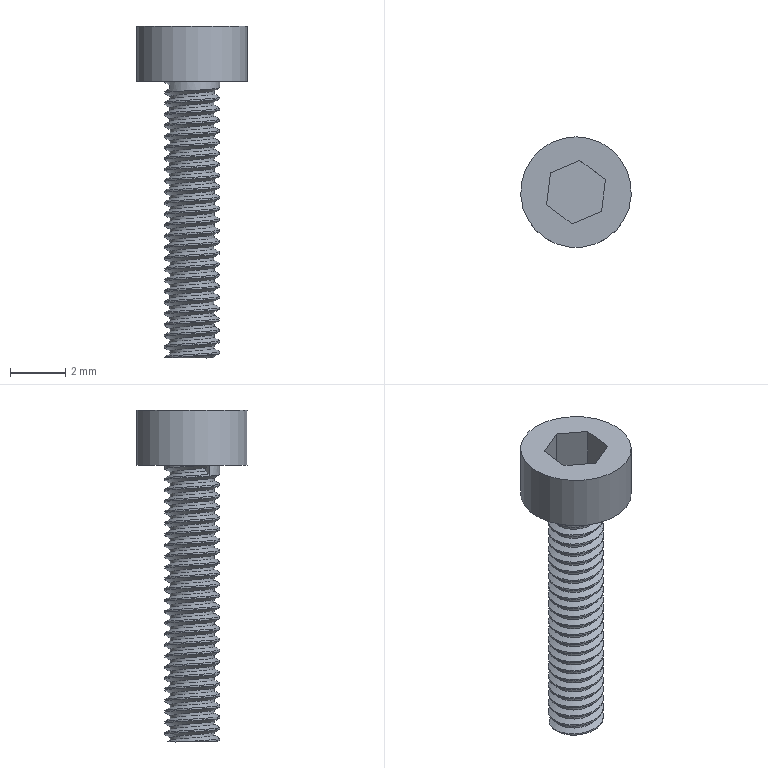Part | NX | features DATUM_CSYS 4, EXTRUDE 3, SKETCH 3, THREADS 1 | 1 solid | 17 faces | box 4 x 4 x 12 mm | volume 45.055 mm3 | plane 11 | cylinder 3 | spline 3 | commonest cylinder face diameters 1.6 x1 2 x1 4 x1